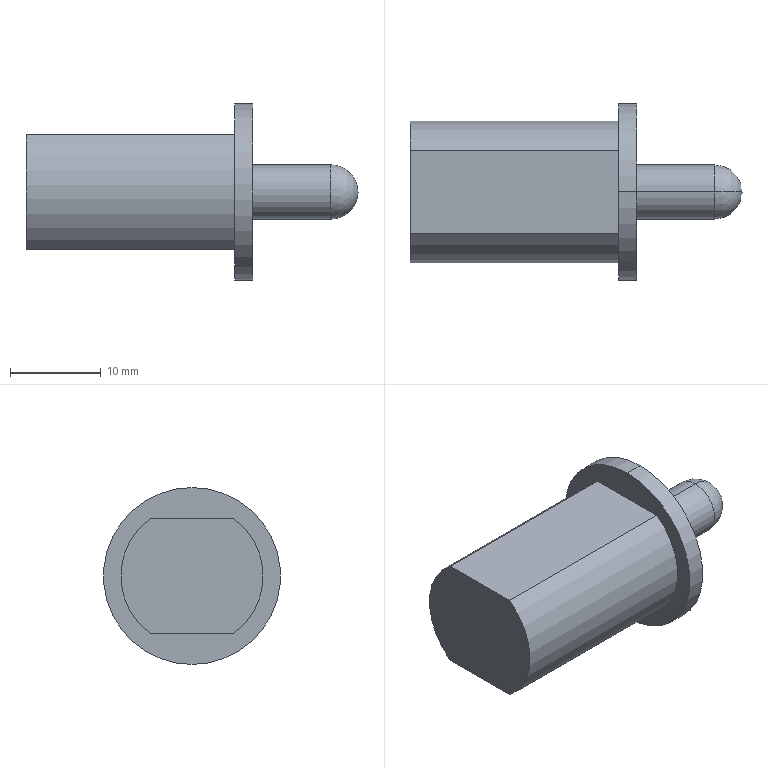Part | STEP file | ZK-0092_160001 | 1 solid | 13 faces | box 36.6 x 19.5 x 19.5 mm | volume 4916 mm3 | cylinder 6 | plane 5 | sphere 2 | commonest cylinder face diameters 6 x2 15.7 x2 19.5 x2
STEP:
#1=CARTESIAN_POINT('',(0.,0.,0.));
#2=DIRECTION('',(0.,0.,1.));
#3=DIRECTION('',(1.,0.,0.));
#4=AXIS2_PLACEMENT_3D('',#1,#2,#3);
#5=CARTESIAN_POINT('',(574.,109.892,1931.35));
#6=VERTEX_POINT('',#5);
#7=CARTESIAN_POINT('',(574.,109.892,1918.65));
#8=VERTEX_POINT('',#7);
#9=CARTESIAN_POINT('',(574.,114.508,1925.));
#10=DIRECTION('',(1.,0.,0.));
#11=DIRECTION('',(0.,-0.5879,0.8089));
#12=AXIS2_PLACEMENT_3D('',#9,#10,#11);
#13=CIRCLE('',#12,7.85);
#14=CARTESIAN_POINT('',(548.,114.508,1925.));
#15=DIRECTION('',(1.,0.,0.));
#16=DIRECTION('',(0.,0.,1.));
#17=AXIS2_PLACEMENT_3D('',#14,#15,#16);
#18=CYLINDRICAL_SURFACE('',#17,7.85);
#19=CARTESIAN_POINT('',(0.6285,26.));
#20=DIRECTION('',(1.,0.));
#21=VECTOR('',#20,1.);
#22=LINE('',#19,#21);
#23=(GEOMETRIC_REPRESENTATION_CONTEXT(2)PARAMETRIC_REPRESENTATION_CONTEXT()REPRESENTATION_CONTEXT('',''));
#24=DEFINITIONAL_REPRESENTATION('',(#22),#23);
#25=PCURVE('',#18,#24);
#26=CARTESIAN_POINT('',(574.,114.508,1925.));
#27=DIRECTION('',(1.,0.,0.));
#28=DIRECTION('',(0.,0.,1.));
#29=AXIS2_PLACEMENT_3D('',#26,#27,#28);
#30=PLANE('',#29);
#31=CARTESIAN_POINT('',(0.,0.));
#32=DIRECTION('',(0.8089,0.5879));
#33=AXIS2_PLACEMENT_2D('',#31,#32);
#34=CIRCLE('',#33,7.85);
#35=(GEOMETRIC_REPRESENTATION_CONTEXT(2)PARAMETRIC_REPRESENTATION_CONTEXT()REPRESENTATION_CONTEXT('',''));
#36=DEFINITIONAL_REPRESENTATION('',(#34),#35);
#37=PCURVE('',#30,#36);
#38=SURFACE_CURVE('',#13,(#25,#37),.PCURVE_S1.);
#39=EDGE_CURVE('',#6,#8,#38,.T.);
#40=ORIENTED_EDGE('',*,*,#39,.F.);
#41=CARTESIAN_POINT('',(551.,109.892,1931.35));
#42=VERTEX_POINT('',#41);
#43=CARTESIAN_POINT('',(574.,109.892,1931.35));
#44=DIRECTION('',(-1.,0.,0.));
#45=VECTOR('',#44,1.);
#46=LINE('',#43,#45);
#47=CARTESIAN_POINT('',(0.6285,26.));
#48=DIRECTION('',(0.,-1.));
#49=VECTOR('',#48,1.);
#50=LINE('',#47,#49);
#51=(GEOMETRIC_REPRESENTATION_CONTEXT(2)PARAMETRIC_REPRESENTATION_CONTEXT()REPRESENTATION_CONTEXT('',''));
#52=DEFINITIONAL_REPRESENTATION('',(#50),#51);
#53=PCURVE('',#18,#52);
#54=CARTESIAN_POINT('',(561.,128.108,1931.35));
#55=DIRECTION('',(0.,0.,-1.));
#56=DIRECTION('',(1.,0.,0.));
#57=AXIS2_PLACEMENT_3D('',#54,#55,#56);
#58=PLANE('',#57);
#59=CARTESIAN_POINT('',(13.,18.215));
#60=DIRECTION('',(-1.,0.));
#61=VECTOR('',#60,1.);
#62=LINE('',#59,#61);
#63=(GEOMETRIC_REPRESENTATION_CONTEXT(2)PARAMETRIC_REPRESENTATION_CONTEXT()REPRESENTATION_CONTEXT('',''));
#64=DEFINITIONAL_REPRESENTATION('',(#62),#63);
#65=PCURVE('',#58,#64);
#66=SURFACE_CURVE('',#46,(#53,#65),.PCURVE_S1.);
#67=EDGE_CURVE('',#6,#42,#66,.T.);
#68=ORIENTED_EDGE('',*,*,#67,.T.);
#69=CARTESIAN_POINT('',(551.,109.892,1918.65));
#70=VERTEX_POINT('',#69);
#71=CARTESIAN_POINT('',(551.,114.508,1925.));
#72=DIRECTION('',(-1.,0.,0.));
#73=DIRECTION('',(0.,-0.5879,-0.8089));
#74=AXIS2_PLACEMENT_3D('',#71,#72,#73);
#75=CIRCLE('',#74,7.85);
#76=CARTESIAN_POINT('',(2.513,3.));
#77=DIRECTION('',(-1.,0.));
#78=VECTOR('',#77,1.);
#79=LINE('',#76,#78);
#80=(GEOMETRIC_REPRESENTATION_CONTEXT(2)PARAMETRIC_REPRESENTATION_CONTEXT()REPRESENTATION_CONTEXT('',''));
#81=DEFINITIONAL_REPRESENTATION('',(#79),#80);
#82=PCURVE('',#18,#81);
#83=CARTESIAN_POINT('',(551.,114.508,1925.));
#84=DIRECTION('',(-1.,0.,0.));
#85=DIRECTION('',(0.,0.,-1.));
#86=AXIS2_PLACEMENT_3D('',#83,#84,#85);
#87=PLANE('',#86);
#88=CARTESIAN_POINT('',(0.,0.));
#89=DIRECTION('',(0.8089,0.5879));
#90=AXIS2_PLACEMENT_2D('',#88,#89);
#91=CIRCLE('',#90,7.85);
#92=(GEOMETRIC_REPRESENTATION_CONTEXT(2)PARAMETRIC_REPRESENTATION_CONTEXT()REPRESENTATION_CONTEXT('',''));
#93=DEFINITIONAL_REPRESENTATION('',(#91),#92);
#94=PCURVE('',#87,#93);
#95=SURFACE_CURVE('',#75,(#82,#94),.PCURVE_S1.);
#96=EDGE_CURVE('',#70,#42,#95,.T.);
#97=ORIENTED_EDGE('',*,*,#96,.F.);
#98=CARTESIAN_POINT('',(551.,109.892,1918.65));
#99=DIRECTION('',(1.,0.,0.));
#100=VECTOR('',#99,1.);
#101=LINE('',#98,#100);
#102=CARTESIAN_POINT('',(2.513,3.));
#103=DIRECTION('',(0.,1.));
#104=VECTOR('',#103,1.);
#105=LINE('',#102,#104);
#106=(GEOMETRIC_REPRESENTATION_CONTEXT(2)PARAMETRIC_REPRESENTATION_CONTEXT()REPRESENTATION_CONTEXT('',''));
#107=DEFINITIONAL_REPRESENTATION('',(#105),#106);
#108=PCURVE('',#18,#107);
#109=CARTESIAN_POINT('',(561.,101.108,1918.65));
#110=DIRECTION('',(0.,0.,1.));
#111=DIRECTION('',(-1.,0.,0.));
#112=AXIS2_PLACEMENT_3D('',#109,#110,#111);
#113=PLANE('',#112);
#114=CARTESIAN_POINT('',(10.,-8.785));
#115=DIRECTION('',(-1.,0.));
#116=VECTOR('',#115,1.);
#117=LINE('',#114,#116);
#118=(GEOMETRIC_REPRESENTATION_CONTEXT(2)PARAMETRIC_REPRESENTATION_CONTEXT()REPRESENTATION_CONTEXT('',''));
#119=DEFINITIONAL_REPRESENTATION('',(#117),#118);
#120=PCURVE('',#113,#119);
#121=SURFACE_CURVE('',#101,(#108,#120),.PCURVE_S1.);
#122=EDGE_CURVE('',#70,#8,#121,.T.);
#123=ORIENTED_EDGE('',*,*,#122,.T.);
#124=EDGE_LOOP('',(#40,#68,#97,#123));
#125=FACE_BOUND('',#124,.T.);
#126=ADVANCED_FACE('',(#125),#18,.T.);
#127=CARTESIAN_POINT('',(551.,119.123,1918.65));
#128=VERTEX_POINT('',#127);
#129=CARTESIAN_POINT('',(551.,119.123,1918.65));
#130=DIRECTION('',(0.,-1.,0.));
#131=VECTOR('',#130,1.);
#132=LINE('',#129,#131);
#133=CARTESIAN_POINT('',(10.,-18.015));
#134=DIRECTION('',(0.,1.));
#135=VECTOR('',#134,1.);
#136=LINE('',#133,#135);
#137=(GEOMETRIC_REPRESENTATION_CONTEXT(2)PARAMETRIC_REPRESENTATION_CONTEXT()REPRESENTATION_CONTEXT('',''));
#138=DEFINITIONAL_REPRESENTATION('',(#136),#137);
#139=PCURVE('',#113,#138);
#140=CARTESIAN_POINT('',(6.35,-4.615));
#141=DIRECTION('',(0.,1.));
#142=VECTOR('',#141,1.);
#143=LINE('',#140,#142);
#144=(GEOMETRIC_REPRESENTATION_CONTEXT(2)PARAMETRIC_REPRESENTATION_CONTEXT()REPRESENTATION_CONTEXT('',''));
#145=DEFINITIONAL_REPRESENTATION('',(#143),#144);
#146=PCURVE('',#87,#145);
#147=SURFACE_CURVE('',#132,(#139,#146),.PCURVE_S1.);
#148=EDGE_CURVE('',#128,#70,#147,.T.);
#149=ORIENTED_EDGE('',*,*,#148,.T.);
#150=ORIENTED_EDGE('',*,*,#122,.T.);
#151=CARTESIAN_POINT('',(574.,119.123,1918.65));
#152=VERTEX_POINT('',#151);
#153=CARTESIAN_POINT('',(574.,109.892,1918.65));
#154=DIRECTION('',(0.,1.,0.));
#155=VECTOR('',#154,1.);
#156=LINE('',#153,#155);
#157=CARTESIAN_POINT('',(-13.,-8.785));
#158=DIRECTION('',(0.,-1.));
#159=VECTOR('',#158,1.);
#160=LINE('',#157,#159);
#161=(GEOMETRIC_REPRESENTATION_CONTEXT(2)PARAMETRIC_REPRESENTATION_CONTEXT()REPRESENTATION_CONTEXT('',''));
#162=DEFINITIONAL_REPRESENTATION('',(#160),#161);
#163=PCURVE('',#113,#162);
#164=CARTESIAN_POINT('',(-6.35,4.615));
#165=DIRECTION('',(0.,-1.));
#166=VECTOR('',#165,1.);
#167=LINE('',#164,#166);
#168=(GEOMETRIC_REPRESENTATION_CONTEXT(2)PARAMETRIC_REPRESENTATION_CONTEXT()REPRESENTATION_CONTEXT('',''));
#169=DEFINITIONAL_REPRESENTATION('',(#167),#168);
#170=PCURVE('',#30,#169);
#171=SURFACE_CURVE('',#156,(#163,#170),.PCURVE_S1.);
#172=EDGE_CURVE('',#8,#152,#171,.T.);
#173=ORIENTED_EDGE('',*,*,#172,.T.);
#174=CARTESIAN_POINT('',(574.,119.123,1918.65));
#175=DIRECTION('',(-1.,0.,0.));
#176=VECTOR('',#175,1.);
#177=LINE('',#174,#176);
#178=CARTESIAN_POINT('',(-13.,-18.015));
#179=DIRECTION('',(1.,0.));
#180=VECTOR('',#179,1.);
#181=LINE('',#178,#180);
#182=(GEOMETRIC_REPRESENTATION_CONTEXT(2)PARAMETRIC_REPRESENTATION_CONTEXT()REPRESENTATION_CONTEXT('',''));
#183=DEFINITIONAL_REPRESENTATION('',(#181),#182);
#184=PCURVE('',#113,#183);
#185=CARTESIAN_POINT('',(548.,114.508,1925.));
#186=DIRECTION('',(1.,0.,0.));
#187=DIRECTION('',(0.,0.,1.));
#188=AXIS2_PLACEMENT_3D('',#185,#186,#187);
#189=CYLINDRICAL_SURFACE('',#188,7.85);
#190=CARTESIAN_POINT('',(3.77,26.));
#191=DIRECTION('',(0.,-1.));
#192=VECTOR('',#191,1.);
#193=LINE('',#190,#192);
#194=(GEOMETRIC_REPRESENTATION_CONTEXT(2)PARAMETRIC_REPRESENTATION_CONTEXT()REPRESENTATION_CONTEXT('',''));
#195=DEFINITIONAL_REPRESENTATION('',(#193),#194);
#196=PCURVE('',#189,#195);
#197=SURFACE_CURVE('',#177,(#184,#196),.PCURVE_S1.);
#198=EDGE_CURVE('',#152,#128,#197,.T.);
#199=ORIENTED_EDGE('',*,*,#198,.T.);
#200=EDGE_LOOP('',(#149,#150,#173,#199));
#201=FACE_BOUND('',#200,.F.);
#202=ADVANCED_FACE('',(#201),#113,.F.);
#203=CARTESIAN_POINT('',(551.,119.123,1931.35));
#204=VERTEX_POINT('',#203);
#205=CARTESIAN_POINT('',(551.,109.892,1931.35));
#206=DIRECTION('',(0.,1.,0.));
#207=VECTOR('',#206,1.);
#208=LINE('',#205,#207);
#209=CARTESIAN_POINT('',(-6.35,4.615));
#210=DIRECTION('',(0.,-1.));
#211=VECTOR('',#210,1.);
#212=LINE('',#209,#211);
#213=(GEOMETRIC_REPRESENTATION_CONTEXT(2)PARAMETRIC_REPRESENTATION_CONTEXT()REPRESENTATION_CONTEXT('',''));
#214=DEFINITIONAL_REPRESENTATION('',(#212),#213);
#215=PCURVE('',#87,#214);
#216=CARTESIAN_POINT('',(-10.,18.215));
#217=DIRECTION('',(0.,-1.));
#218=VECTOR('',#217,1.);
#219=LINE('',#216,#218);
#220=(GEOMETRIC_REPRESENTATION_CONTEXT(2)PARAMETRIC_REPRESENTATION_CONTEXT()REPRESENTATION_CONTEXT('',''));
#221=DEFINITIONAL_REPRESENTATION('',(#219),#220);
#222=PCURVE('',#58,#221);
#223=SURFACE_CURVE('',#208,(#215,#222),.PCURVE_S1.);
#224=EDGE_CURVE('',#42,#204,#223,.T.);
#225=ORIENTED_EDGE('',*,*,#224,.F.);
#226=ORIENTED_EDGE('',*,*,#96,.F.);
#227=ORIENTED_EDGE('',*,*,#148,.F.);
#228=CARTESIAN_POINT('',(551.,114.508,1925.));
#229=DIRECTION('',(-1.,0.,0.));
#230=DIRECTION('',(0.,0.5879,0.8089));
#231=AXIS2_PLACEMENT_3D('',#228,#229,#230);
#232=CIRCLE('',#231,7.85);
#233=CARTESIAN_POINT('',(0.,0.));
#234=DIRECTION('',(-0.8089,-0.5879));
#235=AXIS2_PLACEMENT_2D('',#233,#234);
#236=CIRCLE('',#235,7.85);
#237=(GEOMETRIC_REPRESENTATION_CONTEXT(2)PARAMETRIC_REPRESENTATION_CONTEXT()REPRESENTATION_CONTEXT('',''));
#238=DEFINITIONAL_REPRESENTATION('',(#236),#237);
#239=PCURVE('',#87,#238);
#240=CARTESIAN_POINT('',(5.655,3.));
#241=DIRECTION('',(-1.,0.));
#242=VECTOR('',#241,1.);
#243=LINE('',#240,#242);
#244=(GEOMETRIC_REPRESENTATION_CONTEXT(2)PARAMETRIC_REPRESENTATION_CONTEXT()REPRESENTATION_CONTEXT('',''));
#245=DEFINITIONAL_REPRESENTATION('',(#243),#244);
#246=PCURVE('',#189,#245);
#247=SURFACE_CURVE('',#232,(#239,#246),.PCURVE_S1.);
#248=EDGE_CURVE('',#204,#128,#247,.T.);
#249=ORIENTED_EDGE('',*,*,#248,.F.);
#250=EDGE_LOOP('',(#225,#226,#227,#249));
#251=FACE_BOUND('',#250,.F.);
#252=ADVANCED_FACE('',(#251),#87,.T.);
#253=ORIENTED_EDGE('',*,*,#224,.T.);
#254=CARTESIAN_POINT('',(574.,119.123,1931.35));
#255=VERTEX_POINT('',#254);
#256=CARTESIAN_POINT('',(551.,119.123,1931.35));
#257=DIRECTION('',(1.,0.,0.));
#258=VECTOR('',#257,1.);
#259=LINE('',#256,#258);
#260=CARTESIAN_POINT('',(-10.,8.985));
#261=DIRECTION('',(1.,0.));
#262=VECTOR('',#261,1.);
#263=LINE('',#260,#262);
#264=(GEOMETRIC_REPRESENTATION_CONTEXT(2)PARAMETRIC_REPRESENTATION_CONTEXT()REPRESENTATION_CONTEXT('',''));
#265=DEFINITIONAL_REPRESENTATION('',(#263),#264);
#266=PCURVE('',#58,#265);
#267=CARTESIAN_POINT('',(5.655,3.));
#268=DIRECTION('',(0.,1.));
#269=VECTOR('',#268,1.);
#270=LINE('',#267,#269);
#271=(GEOMETRIC_REPRESENTATION_CONTEXT(2)PARAMETRIC_REPRESENTATION_CONTEXT()REPRESENTATION_CONTEXT('',''));
#272=DEFINITIONAL_REPRESENTATION('',(#270),#271);
#273=PCURVE('',#189,#272);
#274=SURFACE_CURVE('',#259,(#266,#273),.PCURVE_S1.);
#275=EDGE_CURVE('',#204,#255,#274,.T.);
#276=ORIENTED_EDGE('',*,*,#275,.T.);
#277=CARTESIAN_POINT('',(574.,119.123,1931.35));
#278=DIRECTION('',(0.,-1.,0.));
#279=VECTOR('',#278,1.);
#280=LINE('',#277,#279);
#281=CARTESIAN_POINT('',(13.,8.985));
#282=DIRECTION('',(0.,1.));
#283=VECTOR('',#282,1.);
#284=LINE('',#281,#283);
#285=(GEOMETRIC_REPRESENTATION_CONTEXT(2)PARAMETRIC_REPRESENTATION_CONTEXT()REPRESENTATION_CONTEXT('',''));
#286=DEFINITIONAL_REPRESENTATION('',(#284),#285);
#287=PCURVE('',#58,#286);
#288=CARTESIAN_POINT('',(6.35,-4.615));
#289=DIRECTION('',(0.,1.));
#290=VECTOR('',#289,1.);
#291=LINE('',#288,#290);
#292=(GEOMETRIC_REPRESENTATION_CONTEXT(2)PARAMETRIC_REPRESENTATION_CONTEXT()REPRESENTATION_CONTEXT('',''));
#293=DEFINITIONAL_REPRESENTATION('',(#291),#292);
#294=PCURVE('',#30,#293);
#295=SURFACE_CURVE('',#280,(#287,#294),.PCURVE_S1.);
#296=EDGE_CURVE('',#255,#6,#295,.T.);
#297=ORIENTED_EDGE('',*,*,#296,.T.);
#298=ORIENTED_EDGE('',*,*,#67,.T.);
#299=EDGE_LOOP('',(#253,#276,#297,#298));
#300=FACE_BOUND('',#299,.F.);
#301=ADVANCED_FACE('',(#300),#58,.F.);
#302=ORIENTED_EDGE('',*,*,#275,.T.);
#303=CARTESIAN_POINT('',(574.,114.508,1925.));
#304=DIRECTION('',(1.,0.,0.));
#305=DIRECTION('',(0.,0.5879,-0.8089));
#306=AXIS2_PLACEMENT_3D('',#303,#304,#305);
#307=CIRCLE('',#306,7.85);
#308=CARTESIAN_POINT('',(3.77,26.));
#309=DIRECTION('',(1.,0.));
#310=VECTOR('',#309,1.);
#311=LINE('',#308,#310);
#312=(GEOMETRIC_REPRESENTATION_CONTEXT(2)PARAMETRIC_REPRESENTATION_CONTEXT()REPRESENTATION_CONTEXT('',''));
#313=DEFINITIONAL_REPRESENTATION('',(#311),#312);
#314=PCURVE('',#189,#313);
#315=CARTESIAN_POINT('',(0.,0.));
#316=DIRECTION('',(-0.8089,-0.5879));
#317=AXIS2_PLACEMENT_2D('',#315,#316);
#318=CIRCLE('',#317,7.85);
#319=(GEOMETRIC_REPRESENTATION_CONTEXT(2)PARAMETRIC_REPRESENTATION_CONTEXT()REPRESENTATION_CONTEXT('',''));
#320=DEFINITIONAL_REPRESENTATION('',(#318),#319);
#321=PCURVE('',#30,#320);
#322=SURFACE_CURVE('',#307,(#314,#321),.PCURVE_S1.);
#323=EDGE_CURVE('',#152,#255,#322,.T.);
#324=ORIENTED_EDGE('',*,*,#323,.F.);
#325=ORIENTED_EDGE('',*,*,#198,.T.);
#326=ORIENTED_EDGE('',*,*,#248,.F.);
#327=EDGE_LOOP('',(#302,#324,#325,#326));
#328=FACE_BOUND('',#327,.T.);
#329=ADVANCED_FACE('',(#328),#189,.T.);
#330=CARTESIAN_POINT('',(574.,114.508,1915.25));
#331=VERTEX_POINT('',#330);
#332=CARTESIAN_POINT('',(574.,114.508,1934.75));
#333=VERTEX_POINT('',#332);
#334=CARTESIAN_POINT('',(574.,114.508,1925.));
#335=DIRECTION('',(-1.,0.,0.));
#336=DIRECTION('',(0.,0.,-1.));
#337=AXIS2_PLACEMENT_3D('',#334,#335,#336);
#338=CIRCLE('',#337,9.75);
#339=CARTESIAN_POINT('',(-9.75,0.));
#340=CARTESIAN_POINT('',(-9.75,16.887));
#341=CARTESIAN_POINT('',(4.875,8.444));
#342=CARTESIAN_POINT('',(19.5,0.));
#343=CARTESIAN_POINT('',(4.875,-8.444));
#344=CARTESIAN_POINT('',(-9.75,-16.887));
#345=CARTESIAN_POINT('',(-9.75,0.));
#346=(BOUNDED_CURVE()B_SPLINE_CURVE(2,(#339,#340,#341,#342,#343,#344,#345),.UNSPECIFIED.,.T.,.F.)B_SPLINE_CURVE_WITH_KNOTS((1,2,2,2,2,1),(-2.094,0.,2.094,4.189,6.283,8.378),.UNSPECIFIED.)CURVE()GEOMETRIC_REPRESENTATION_ITEM()RATIONAL_B_SPLINE_CURVE((1.,0.5,1.,0.5,1.,0.5,1.))REPRESENTATION_ITEM(''));
#347=(GEOMETRIC_REPRESENTATION_CONTEXT(2)PARAMETRIC_REPRESENTATION_CONTEXT()REPRESENTATION_CONTEXT('',''));
#348=DEFINITIONAL_REPRESENTATION('',(#346),#347);
#349=PCURVE('',#30,#348);
#350=CARTESIAN_POINT('',(576.,114.508,1925.));
#351=DIRECTION('',(-1.,0.,0.));
#352=DIRECTION('',(0.,0.,-1.));
#353=AXIS2_PLACEMENT_3D('',#350,#351,#352);
#354=CYLINDRICAL_SURFACE('',#353,9.75);
#355=CARTESIAN_POINT('',(0.,2.));
#356=DIRECTION('',(1.,0.));
#357=VECTOR('',#356,1.);
#358=LINE('',#355,#357);
#359=(GEOMETRIC_REPRESENTATION_CONTEXT(2)PARAMETRIC_REPRESENTATION_CONTEXT()REPRESENTATION_CONTEXT('',''));
#360=DEFINITIONAL_REPRESENTATION('',(#358),#359);
#361=PCURVE('',#354,#360);
#362=SURFACE_CURVE('',#338,(#349,#361),.PCURVE_S1.);
#363=EDGE_CURVE('',#331,#333,#362,.T.);
#364=ORIENTED_EDGE('',*,*,#363,.F.);
#365=CARTESIAN_POINT('',(574.,114.508,1925.));
#366=DIRECTION('',(-1.,0.,0.));
#367=DIRECTION('',(0.,0.,1.));
#368=AXIS2_PLACEMENT_3D('',#365,#366,#367);
#369=CIRCLE('',#368,9.75);
#370=CARTESIAN_POINT('',(9.75,0.));
#371=CARTESIAN_POINT('',(9.75,-16.887));
#372=CARTESIAN_POINT('',(-4.875,-8.444));
#373=CARTESIAN_POINT('',(-19.5,0.));
#374=CARTESIAN_POINT('',(-4.875,8.444));
#375=CARTESIAN_POINT('',(9.75,16.887));
#376=CARTESIAN_POINT('',(9.75,0.));
#377=(BOUNDED_CURVE()B_SPLINE_CURVE(2,(#370,#371,#372,#373,#374,#375,#376),.UNSPECIFIED.,.T.,.F.)B_SPLINE_CURVE_WITH_KNOTS((1,2,2,2,2,1),(-2.094,0.,2.094,4.189,6.283,8.378),.UNSPECIFIED.)CURVE()GEOMETRIC_REPRESENTATION_ITEM()RATIONAL_B_SPLINE_CURVE((1.,0.5,1.,0.5,1.,0.5,1.))REPRESENTATION_ITEM(''));
#378=(GEOMETRIC_REPRESENTATION_CONTEXT(2)PARAMETRIC_REPRESENTATION_CONTEXT()REPRESENTATION_CONTEXT('',''));
#379=DEFINITIONAL_REPRESENTATION('',(#377),#378);
#380=PCURVE('',#30,#379);
#381=CARTESIAN_POINT('',(576.,114.508,1925.));
#382=DIRECTION('',(-1.,0.,0.));
#383=DIRECTION('',(0.,0.,-1.));
#384=AXIS2_PLACEMENT_3D('',#381,#382,#383);
#385=CYLINDRICAL_SURFACE('',#384,9.75);
#386=CARTESIAN_POINT('',(3.142,2.));
#387=DIRECTION('',(1.,0.));
#388=VECTOR('',#387,1.);
#389=LINE('',#386,#388);
#390=(GEOMETRIC_REPRESENTATION_CONTEXT(2)PARAMETRIC_REPRESENTATION_CONTEXT()REPRESENTATION_CONTEXT('',''));
#391=DEFINITIONAL_REPRESENTATION('',(#389),#390);
#392=PCURVE('',#385,#391);
#393=SURFACE_CURVE('',#369,(#380,#392),.PCURVE_S1.);
#394=EDGE_CURVE('',#333,#331,#393,.T.);
#395=ORIENTED_EDGE('',*,*,#394,.F.);
#396=EDGE_LOOP('',(#364,#395));
#397=FACE_BOUND('',#396,.F.);
#398=ORIENTED_EDGE('',*,*,#323,.F.);
#399=ORIENTED_EDGE('',*,*,#172,.F.);
#400=ORIENTED_EDGE('',*,*,#39,.F.);
#401=ORIENTED_EDGE('',*,*,#296,.F.);
#402=EDGE_LOOP('',(#398,#399,#400,#401));
#403=FACE_BOUND('',#402,.F.);
#404=ADVANCED_FACE('',(#397,#403),#30,.F.);
#405=CARTESIAN_POINT('',(576.,114.508,1934.75));
#406=VERTEX_POINT('',#405);
#407=CARTESIAN_POINT('',(576.,114.508,1934.75));
#408=DIRECTION('',(-1.,0.,0.));
#409=VECTOR('',#408,1.);
#410=LINE('',#407,#409);
#411=CARTESIAN_POINT('',(3.142,0.));
#412=DIRECTION('',(0.,1.));
#413=VECTOR('',#412,1.);
#414=LINE('',#411,#413);
#415=(GEOMETRIC_REPRESENTATION_CONTEXT(2)PARAMETRIC_REPRESENTATION_CONTEXT()REPRESENTATION_CONTEXT('',''));
#416=DEFINITIONAL_REPRESENTATION('',(#414),#415);
#417=PCURVE('',#354,#416);
#418=CARTESIAN_POINT('',(3.142,0.));
#419=DIRECTION('',(0.,1.));
#420=VECTOR('',#419,1.);
#421=LINE('',#418,#420);
#422=(GEOMETRIC_REPRESENTATION_CONTEXT(2)PARAMETRIC_REPRESENTATION_CONTEXT()REPRESENTATION_CONTEXT('',''));
#423=DEFINITIONAL_REPRESENTATION('',(#421),#422);
#424=PCURVE('',#385,#423);
#425=SURFACE_CURVE('',#410,(#417,#424),.PCURVE_S1.);
#426=EDGE_CURVE('',#406,#333,#425,.T.);
#427=ORIENTED_EDGE('',*,*,#426,.T.);
#428=ORIENTED_EDGE('',*,*,#363,.F.);
#429=CARTESIAN_POINT('',(576.,114.508,1915.25));
#430=VERTEX_POINT('',#429);
#431=CARTESIAN_POINT('',(576.,114.508,1915.25));
#432=DIRECTION('',(-1.,0.,0.));
#433=VECTOR('',#432,1.);
#434=LINE('',#431,#433);
#435=CARTESIAN_POINT('',(0.,0.));
#436=DIRECTION('',(0.,1.));
#437=VECTOR('',#436,1.);
#438=LINE('',#435,#437);
#439=(GEOMETRIC_REPRESENTATION_CONTEXT(2)PARAMETRIC_REPRESENTATION_CONTEXT()REPRESENTATION_CONTEXT('',''));
#440=DEFINITIONAL_REPRESENTATION('',(#438),#439);
#441=PCURVE('',#354,#440);
#442=CARTESIAN_POINT('',(6.283,0.));
#443=DIRECTION('',(0.,1.));
#444=VECTOR('',#443,1.);
#445=LINE('',#442,#444);
#446=(GEOMETRIC_REPRESENTATION_CONTEXT(2)PARAMETRIC_REPRESENTATION_CONTEXT()REPRESENTATION_CONTEXT('',''));
#447=DEFINITIONAL_REPRESENTATION('',(#445),#446);
#448=PCURVE('',#385,#447);
#449=SURFACE_CURVE('',#434,(#441,#448),.PCURVE_S1.);
#450=EDGE_CURVE('',#430,#331,#449,.T.);
#451=ORIENTED_EDGE('',*,*,#450,.F.);
#452=CARTESIAN_POINT('',(576.,114.508,1925.));
#453=DIRECTION('',(1.,0.,0.));
#454=DIRECTION('',(0.,0.,1.));
#455=AXIS2_PLACEMENT_3D('',#452,#453,#454);
#456=CIRCLE('',#455,9.75);
#457=CARTESIAN_POINT('',(3.142,0.));
#458=DIRECTION('',(-1.,0.));
#459=VECTOR('',#458,1.);
#460=LINE('',#457,#459);
#461=(GEOMETRIC_REPRESENTATION_CONTEXT(2)PARAMETRIC_REPRESENTATION_CONTEXT()REPRESENTATION_CONTEXT('',''));
#462=DEFINITIONAL_REPRESENTATION('',(#460),#461);
#463=PCURVE('',#354,#462);
#464=CARTESIAN_POINT('',(576.,114.508,1925.));
#465=DIRECTION('',(1.,0.,0.));
#466=DIRECTION('',(0.,0.,1.));
#467=AXIS2_PLACEMENT_3D('',#464,#465,#466);
#468=PLANE('',#467);
#469=CARTESIAN_POINT('',(0.,0.));
#470=DIRECTION('',(1.,0.));
#471=AXIS2_PLACEMENT_2D('',#469,#470);
#472=CIRCLE('',#471,9.75);
#473=(GEOMETRIC_REPRESENTATION_CONTEXT(2)PARAMETRIC_REPRESENTATION_CONTEXT()REPRESENTATION_CONTEXT('',''));
#474=DEFINITIONAL_REPRESENTATION('',(#472),#473);
#475=PCURVE('',#468,#474);
#476=SURFACE_CURVE('',#456,(#463,#475),.PCURVE_S1.);
#477=EDGE_CURVE('',#406,#430,#476,.T.);
#478=ORIENTED_EDGE('',*,*,#477,.F.);
#479=EDGE_LOOP('',(#427,#428,#451,#478));
#480=FACE_BOUND('',#479,.T.);
#481=ADVANCED_FACE('',(#480),#354,.T.);
#482=CARTESIAN_POINT('',(576.,114.508,1925.));
#483=DIRECTION('',(1.,0.,0.));
#484=DIRECTION('',(0.,0.,-1.));
#485=AXIS2_PLACEMENT_3D('',#482,#483,#484);
#486=CIRCLE('',#485,9.75);
#487=CARTESIAN_POINT('',(0.,0.));
#488=DIRECTION('',(-1.,0.));
#489=AXIS2_PLACEMENT_2D('',#487,#488);
#490=CIRCLE('',#489,9.75);
#491=(GEOMETRIC_REPRESENTATION_CONTEXT(2)PARAMETRIC_REPRESENTATION_CONTEXT()REPRESENTATION_CONTEXT('',''));
#492=DEFINITIONAL_REPRESENTATION('',(#490),#491);
#493=PCURVE('',#468,#492);
#494=CARTESIAN_POINT('',(6.283,0.));
#495=DIRECTION('',(-1.,0.));
#496=VECTOR('',#495,1.);
#497=LINE('',#494,#496);
#498=(GEOMETRIC_REPRESENTATION_CONTEXT(2)PARAMETRIC_REPRESENTATION_CONTEXT()REPRESENTATION_CONTEXT('',''));
#499=DEFINITIONAL_REPRESENTATION('',(#497),#498);
#500=PCURVE('',#385,#499);
#501=SURFACE_CURVE('',#486,(#493,#500),.PCURVE_S1.);
#502=EDGE_CURVE('',#430,#406,#501,.T.);
#503=ORIENTED_EDGE('',*,*,#502,.F.);
#504=ORIENTED_EDGE('',*,*,#477,.F.);
#505=EDGE_LOOP('',(#503,#504));
#506=FACE_BOUND('',#505,.F.);
#507=CARTESIAN_POINT('',(576.,114.508,1922.));
#508=VERTEX_POINT('',#507);
#509=CARTESIAN_POINT('',(576.,114.508,1928.));
#510=VERTEX_POINT('',#509);
#511=CARTESIAN_POINT('',(576.,114.508,1925.));
#512=DIRECTION('',(-1.,0.,0.));
#513=DIRECTION('',(0.,0.,-1.));
#514=AXIS2_PLACEMENT_3D('',#511,#512,#513);
#515=CIRCLE('',#514,3.);
#516=CARTESIAN_POINT('',(-3.,0.));
#517=CARTESIAN_POINT('',(-3.,5.196));
#518=CARTESIAN_POINT('',(1.5,2.598));
#519=CARTESIAN_POINT('',(6.,0.));
#520=CARTESIAN_POINT('',(1.5,-2.598));
#521=CARTESIAN_POINT('',(-3.,-5.196));
#522=CARTESIAN_POINT('',(-3.,0.));
#523=(BOUNDED_CURVE()B_SPLINE_CURVE(2,(#516,#517,#518,#519,#520,#521,#522),.UNSPECIFIED.,.T.,.F.)B_SPLINE_CURVE_WITH_KNOTS((1,2,2,2,2,1),(-2.094,0.,2.094,4.189,6.283,8.378),.UNSPECIFIED.)CURVE()GEOMETRIC_REPRESENTATION_ITEM()RATIONAL_B_SPLINE_CURVE((1.,0.5,1.,0.5,1.,0.5,1.))REPRESENTATION_ITEM(''));
#524=(GEOMETRIC_REPRESENTATION_CONTEXT(2)PARAMETRIC_REPRESENTATION_CONTEXT()REPRESENTATION_CONTEXT('',''));
#525=DEFINITIONAL_REPRESENTATION('',(#523),#524);
#526=PCURVE('',#468,#525);
#527=CARTESIAN_POINT('',(587.,114.508,1925.));
#528=DIRECTION('',(-1.,0.,0.));
#529=DIRECTION('',(0.,0.,-1.));
#530=AXIS2_PLACEMENT_3D('',#527,#528,#529);
#531=CYLINDRICAL_SURFACE('',#530,3.);
#532=CARTESIAN_POINT('',(0.,11.));
#533=DIRECTION('',(1.,0.));
#534=VECTOR('',#533,1.);
#535=LINE('',#532,#534);
#536=(GEOMETRIC_REPRESENTATION_CONTEXT(2)PARAMETRIC_REPRESENTATION_CONTEXT()REPRESENTATION_CONTEXT('',''));
#537=DEFINITIONAL_REPRESENTATION('',(#535),#536);
#538=PCURVE('',#531,#537);
#539=SURFACE_CURVE('',#515,(#526,#538),.PCURVE_S1.);
#540=EDGE_CURVE('',#508,#510,#539,.T.);
#541=ORIENTED_EDGE('',*,*,#540,.F.);
#542=CARTESIAN_POINT('',(576.,114.508,1925.));
#543=DIRECTION('',(-1.,0.,0.));
#544=DIRECTION('',(0.,0.,1.));
#545=AXIS2_PLACEMENT_3D('',#542,#543,#544);
#546=CIRCLE('',#545,3.);
#547=CARTESIAN_POINT('',(3.,0.));
#548=CARTESIAN_POINT('',(3.,-5.196));
#549=CARTESIAN_POINT('',(-1.5,-2.598));
#550=CARTESIAN_POINT('',(-6.,0.));
#551=CARTESIAN_POINT('',(-1.5,2.598));
#552=CARTESIAN_POINT('',(3.,5.196));
#553=CARTESIAN_POINT('',(3.,0.));
#554=(BOUNDED_CURVE()B_SPLINE_CURVE(2,(#547,#548,#549,#550,#551,#552,#553),.UNSPECIFIED.,.T.,.F.)B_SPLINE_CURVE_WITH_KNOTS((1,2,2,2,2,1),(-2.094,0.,2.094,4.189,6.283,8.378),.UNSPECIFIED.)CURVE()GEOMETRIC_REPRESENTATION_ITEM()RATIONAL_B_SPLINE_CURVE((1.,0.5,1.,0.5,1.,0.5,1.))REPRESENTATION_ITEM(''));
#555=(GEOMETRIC_REPRESENTATION_CONTEXT(2)PARAMETRIC_REPRESENTATION_CONTEXT()REPRESENTATION_CONTEXT('',''));
#556=DEFINITIONAL_REPRESENTATION('',(#554),#555);
#557=PCURVE('',#468,#556);
#558=CARTESIAN_POINT('',(587.,114.508,1925.));
#559=DIRECTION('',(-1.,0.,0.));
#560=DIRECTION('',(0.,0.,-1.));
#561=AXIS2_PLACEMENT_3D('',#558,#559,#560);
#562=CYLINDRICAL_SURFACE('',#561,3.);
#563=CARTESIAN_POINT('',(3.142,11.));
#564=DIRECTION('',(1.,0.));
#565=VECTOR('',#564,1.);
#566=LINE('',#563,#565);
#567=(GEOMETRIC_REPRESENTATION_CONTEXT(2)PARAMETRIC_REPRESENTATION_CONTEXT()REPRESENTATION_CONTEXT('',''));
#568=DEFINITIONAL_REPRESENTATION('',(#566),#567);
#569=PCURVE('',#562,#568);
#570=SURFACE_CURVE('',#546,(#557,#569),.PCURVE_S1.);
#571=EDGE_CURVE('',#510,#508,#570,.T.);
#572=ORIENTED_EDGE('',*,*,#571,.F.);
#573=EDGE_LOOP('',(#541,#572));
#574=FACE_BOUND('',#573,.F.);
#575=ADVANCED_FACE('',(#506,#574),#468,.T.);
#576=CARTESIAN_POINT('',(584.6,114.508,1928.));
#577=VERTEX_POINT('',#576);
#578=CARTESIAN_POINT('',(584.6,114.508,1928.));
#579=DIRECTION('',(-1.,0.,0.));
#580=VECTOR('',#579,1.);
#581=LINE('',#578,#580);
#582=CARTESIAN_POINT('',(3.142,2.4));
#583=DIRECTION('',(0.,1.));
#584=VECTOR('',#583,1.);
#585=LINE('',#582,#584);
#586=(GEOMETRIC_REPRESENTATION_CONTEXT(2)PARAMETRIC_REPRESENTATION_CONTEXT()REPRESENTATION_CONTEXT('',''));
#587=DEFINITIONAL_REPRESENTATION('',(#585),#586);
#588=PCURVE('',#531,#587);
#589=CARTESIAN_POINT('',(3.142,2.4));
#590=DIRECTION('',(0.,1.));
#591=VECTOR('',#590,1.);
#592=LINE('',#589,#591);
#593=(GEOMETRIC_REPRESENTATION_CONTEXT(2)PARAMETRIC_REPRESENTATION_CONTEXT()REPRESENTATION_CONTEXT('',''));
#594=DEFINITIONAL_REPRESENTATION('',(#592),#593);
#595=PCURVE('',#562,#594);
#596=SURFACE_CURVE('',#581,(#588,#595),.PCURVE_S1.);
#597=EDGE_CURVE('',#577,#510,#596,.T.);
#598=ORIENTED_EDGE('',*,*,#597,.T.);
#599=ORIENTED_EDGE('',*,*,#540,.F.);
#600=CARTESIAN_POINT('',(584.6,114.508,1922.));
#601=VERTEX_POINT('',#600);
#602=CARTESIAN_POINT('',(584.6,114.508,1922.));
#603=DIRECTION('',(-1.,0.,0.));
#604=VECTOR('',#603,1.);
#605=LINE('',#602,#604);
#606=CARTESIAN_POINT('',(0.,2.4));
#607=DIRECTION('',(0.,1.));
#608=VECTOR('',#607,1.);
#609=LINE('',#606,#608);
#610=(GEOMETRIC_REPRESENTATION_CONTEXT(2)PARAMETRIC_REPRESENTATION_CONTEXT()REPRESENTATION_CONTEXT('',''));
#611=DEFINITIONAL_REPRESENTATION('',(#609),#610);
#612=PCURVE('',#531,#611);
#613=CARTESIAN_POINT('',(6.283,2.4));
#614=DIRECTION('',(0.,1.));
#615=VECTOR('',#614,1.);
#616=LINE('',#613,#615);
#617=(GEOMETRIC_REPRESENTATION_CONTEXT(2)PARAMETRIC_REPRESENTATION_CONTEXT()REPRESENTATION_CONTEXT('',''));
#618=DEFINITIONAL_REPRESENTATION('',(#616),#617);
#619=PCURVE('',#562,#618);
#620=SURFACE_CURVE('',#605,(#612,#619),.PCURVE_S1.);
#621=EDGE_CURVE('',#601,#508,#620,.T.);
#622=ORIENTED_EDGE('',*,*,#621,.F.);
#623=CARTESIAN_POINT('',(584.6,114.508,1925.));
#624=DIRECTION('',(1.,0.,0.));
#625=DIRECTION('',(0.,0.,1.));
#626=AXIS2_PLACEMENT_3D('',#623,#624,#625);
#627=CIRCLE('',#626,3.);
#628=CARTESIAN_POINT('',(3.142,2.4));
#629=DIRECTION('',(-1.,0.));
#630=VECTOR('',#629,1.);
#631=LINE('',#628,#630);
#632=(GEOMETRIC_REPRESENTATION_CONTEXT(2)PARAMETRIC_REPRESENTATION_CONTEXT()REPRESENTATION_CONTEXT('',''));
#633=DEFINITIONAL_REPRESENTATION('',(#631),#632);
#634=PCURVE('',#531,#633);
#635=CARTESIAN_POINT('',(584.6,114.508,1925.));
#636=DIRECTION('',(1.,0.,0.));
#637=DIRECTION('',(0.,0.,1.));
#638=AXIS2_PLACEMENT_3D('',#635,#636,#637);
#639=SPHERICAL_SURFACE('',#638,3.);
#640=CARTESIAN_POINT('',(0.,0.));
#641=DIRECTION('',(1.,0.));
#642=VECTOR('',#641,1.);
#643=LINE('',#640,#642);
#644=(GEOMETRIC_REPRESENTATION_CONTEXT(2)PARAMETRIC_REPRESENTATION_CONTEXT()REPRESENTATION_CONTEXT('',''));
#645=DEFINITIONAL_REPRESENTATION('',(#643),#644);
#646=PCURVE('',#639,#645);
#647=SURFACE_CURVE('',#627,(#634,#646),.PCURVE_S1.);
#648=EDGE_CURVE('',#577,#601,#647,.T.);
#649=ORIENTED_EDGE('',*,*,#648,.F.);
#650=EDGE_LOOP('',(#598,#599,#622,#649));
#651=FACE_BOUND('',#650,.T.);
#652=ADVANCED_FACE('',(#651),#531,.T.);
#653=CARTESIAN_POINT('',(587.6,114.508,1925.));
#654=VERTEX_POINT('',#653);
#655=CARTESIAN_POINT('',(584.6,114.508,1925.));
#656=DIRECTION('',(0.,-1.,0.));
#657=DIRECTION('',(0.,0.,-1.));
#658=AXIS2_PLACEMENT_3D('',#655,#656,#657);
#659=CIRCLE('',#658,3.);
#660=CARTESIAN_POINT('',(3.142,0.));
#661=CARTESIAN_POINT('',(3.142,0.0238));
#662=CARTESIAN_POINT('',(3.142,0.0714));
#663=CARTESIAN_POINT('',(3.142,0.1428));
#664=CARTESIAN_POINT('',(3.142,0.2142));
#665=CARTESIAN_POINT('',(3.142,0.2856));
#666=CARTESIAN_POINT('',(3.142,0.357));
#667=CARTESIAN_POINT('',(3.142,0.4284));
#668=CARTESIAN_POINT('',(3.142,0.4998));
#669=CARTESIAN_POINT('',(3.142,0.5712));
#670=CARTESIAN_POINT('',(3.142,0.6426));
#671=CARTESIAN_POINT('',(3.142,0.714));
#672=CARTESIAN_POINT('',(3.142,0.7854));
#673=CARTESIAN_POINT('',(3.142,0.8568));
#674=CARTESIAN_POINT('',(3.142,0.9282));
#675=CARTESIAN_POINT('',(3.142,0.9996));
#676=CARTESIAN_POINT('',(3.142,1.071));
#677=CARTESIAN_POINT('',(3.142,1.142));
#678=CARTESIAN_POINT('',(3.142,1.214));
#679=CARTESIAN_POINT('',(3.142,1.285));
#680=CARTESIAN_POINT('',(3.142,1.357));
#681=CARTESIAN_POINT('',(3.142,1.428));
#682=CARTESIAN_POINT('',(3.142,1.499));
#683=CARTESIAN_POINT('',(3.142,1.547));
#684=CARTESIAN_POINT('',(3.142,1.571));
#685=B_SPLINE_CURVE_WITH_KNOTS('',3,(#660,#661,#662,#663,#664,#665,#666,#667,#668,#669,#670,#671,#672,#673,#674,#675,#676,#677,#678,#679,#680,#681,#682,#683,#684),.UNSPECIFIED.,.F.,.F.,(4,1,1,1,1,1,1,1,1,1,1,1,1,1,1,1,1,1,1,1,1,1,4),(0.,0.0714,0.1428,0.2142,0.2856,0.357,0.4284,0.4998,0.5712,0.6426,0.714,0.7854,0.8568,0.9282,0.9996,1.071,1.142,1.214,1.285,1.357,1.428,1.499,1.571),.QUASI_UNIFORM_KNOTS.);
#686=(GEOMETRIC_REPRESENTATION_CONTEXT(2)PARAMETRIC_REPRESENTATION_CONTEXT()REPRESENTATION_CONTEXT('',''));
#687=DEFINITIONAL_REPRESENTATION('',(#685),#686);
#688=PCURVE('',#639,#687);
#689=CARTESIAN_POINT('',(584.6,114.508,1925.));
#690=DIRECTION('',(1.,0.,0.));
#691=DIRECTION('',(0.,0.,1.));
#692=AXIS2_PLACEMENT_3D('',#689,#690,#691);
#693=SPHERICAL_SURFACE('',#692,3.);
#694=CARTESIAN_POINT('',(3.142,0.));
#695=CARTESIAN_POINT('',(3.142,0.0238));
#696=CARTESIAN_POINT('',(3.142,0.0714));
#697=CARTESIAN_POINT('',(3.142,0.1428));
#698=CARTESIAN_POINT('',(3.142,0.2142));
#699=CARTESIAN_POINT('',(3.142,0.2856));
#700=CARTESIAN_POINT('',(3.142,0.357));
#701=CARTESIAN_POINT('',(3.142,0.4284));
#702=CARTESIAN_POINT('',(3.142,0.4998));
#703=CARTESIAN_POINT('',(3.142,0.5712));
#704=CARTESIAN_POINT('',(3.142,0.6426));
#705=CARTESIAN_POINT('',(3.142,0.714));
#706=CARTESIAN_POINT('',(3.142,0.7854));
#707=CARTESIAN_POINT('',(3.142,0.8568));
#708=CARTESIAN_POINT('',(3.142,0.9282));
#709=CARTESIAN_POINT('',(3.142,0.9996));
#710=CARTESIAN_POINT('',(3.142,1.071));
#711=CARTESIAN_POINT('',(3.142,1.142));
#712=CARTESIAN_POINT('',(3.142,1.214));
#713=CARTESIAN_POINT('',(3.142,1.285));
#714=CARTESIAN_POINT('',(3.142,1.357));
#715=CARTESIAN_POINT('',(3.142,1.428));
#716=CARTESIAN_POINT('',(3.142,1.499));
#717=CARTESIAN_POINT('',(3.142,1.547));
#718=CARTESIAN_POINT('',(3.142,1.571));
#719=B_SPLINE_CURVE_WITH_KNOTS('',3,(#694,#695,#696,#697,#698,#699,#700,#701,#702,#703,#704,#705,#706,#707,#708,#709,#710,#711,#712,#713,#714,#715,#716,#717,#718),.UNSPECIFIED.,.F.,.F.,(4,1,1,1,1,1,1,1,1,1,1,1,1,1,1,1,1,1,1,1,1,1,4),(0.,0.0714,0.1428,0.2142,0.2856,0.357,0.4284,0.4998,0.5712,0.6426,0.714,0.7854,0.8568,0.9282,0.9996,1.071,1.142,1.214,1.285,1.357,1.428,1.499,1.571),.QUASI_UNIFORM_KNOTS.);
#720=(GEOMETRIC_REPRESENTATION_CONTEXT(2)PARAMETRIC_REPRESENTATION_CONTEXT()REPRESENTATION_CONTEXT('',''));
#721=DEFINITIONAL_REPRESENTATION('',(#719),#720);
#722=PCURVE('',#693,#721);
#723=SURFACE_CURVE('',#659,(#688,#722),.PCURVE_S1.);
#724=EDGE_CURVE('',#601,#654,#723,.T.);
#725=ORIENTED_EDGE('',*,*,#724,.T.);
#726=CARTESIAN_POINT('',(584.6,114.508,1925.));
#727=DIRECTION('',(0.,1.,0.));
#728=DIRECTION('',(0.,0.,1.));
#729=AXIS2_PLACEMENT_3D('',#726,#727,#728);
#730=CIRCLE('',#729,3.);
#731=CARTESIAN_POINT('',(0.,0.));
#732=DIRECTION('',(0.,1.));
#733=VECTOR('',#732,1.);
#734=LINE('',#731,#733);
#735=(GEOMETRIC_REPRESENTATION_CONTEXT(2)PARAMETRIC_REPRESENTATION_CONTEXT()REPRESENTATION_CONTEXT('',''));
#736=DEFINITIONAL_REPRESENTATION('',(#734),#735);
#737=PCURVE('',#639,#736);
#738=CARTESIAN_POINT('',(6.283,0.));
#739=DIRECTION('',(0.,1.));
#740=VECTOR('',#739,1.);
#741=LINE('',#738,#740);
#742=(GEOMETRIC_REPRESENTATION_CONTEXT(2)PARAMETRIC_REPRESENTATION_CONTEXT()REPRESENTATION_CONTEXT('',''));
#743=DEFINITIONAL_REPRESENTATION('',(#741),#742);
#744=PCURVE('',#693,#743);
#745=SURFACE_CURVE('',#730,(#737,#744),.PCURVE_S1.);
#746=EDGE_CURVE('',#577,#654,#745,.T.);
#747=ORIENTED_EDGE('',*,*,#746,.F.);
#748=ORIENTED_EDGE('',*,*,#648,.T.);
#749=EDGE_LOOP('',(#725,#747,#748));
#750=FACE_BOUND('',#749,.T.);
#751=ADVANCED_FACE('',(#750),#639,.T.);
#752=ORIENTED_EDGE('',*,*,#746,.T.);
#753=ORIENTED_EDGE('',*,*,#724,.F.);
#754=CARTESIAN_POINT('',(584.6,114.508,1925.));
#755=DIRECTION('',(1.,0.,0.));
#756=DIRECTION('',(0.,0.,-1.));
#757=AXIS2_PLACEMENT_3D('',#754,#755,#756);
#758=CIRCLE('',#757,3.);
#759=CARTESIAN_POINT('',(3.142,0.));
#760=CARTESIAN_POINT('',(3.189,0.));
#761=CARTESIAN_POINT('',(3.284,0.));
#762=CARTESIAN_POINT('',(3.427,0.));
#763=CARTESIAN_POINT('',(3.57,0.));
#764=CARTESIAN_POINT('',(3.713,0.));
#765=CARTESIAN_POINT('',(3.856,0.));
#766=CARTESIAN_POINT('',(3.998,0.));
#767=CARTESIAN_POINT('',(4.141,0.));
#768=CARTESIAN_POINT('',(4.284,0.));
#769=CARTESIAN_POINT('',(4.427,0.));
#770=CARTESIAN_POINT('',(4.57,0.));
#771=CARTESIAN_POINT('',(4.712,0.));
#772=CARTESIAN_POINT('',(4.855,0.));
#773=CARTESIAN_POINT('',(4.998,0.));
#774=CARTESIAN_POINT('',(5.141,0.));
#775=CARTESIAN_POINT('',(5.284,0.));
#776=CARTESIAN_POINT('',(5.426,0.));
#777=CARTESIAN_POINT('',(5.569,0.));
#778=CARTESIAN_POINT('',(5.712,0.));
#779=CARTESIAN_POINT('',(5.855,0.));
#780=CARTESIAN_POINT('',(5.998,0.));
#781=CARTESIAN_POINT('',(6.14,0.));
#782=CARTESIAN_POINT('',(6.236,0.));
#783=CARTESIAN_POINT('',(6.283,0.));
#784=B_SPLINE_CURVE_WITH_KNOTS('',3,(#759,#760,#761,#762,#763,#764,#765,#766,#767,#768,#769,#770,#771,#772,#773,#774,#775,#776,#777,#778,#779,#780,#781,#782,#783),.UNSPECIFIED.,.F.,.F.,(4,1,1,1,1,1,1,1,1,1,1,1,1,1,1,1,1,1,1,1,1,1,4),(0.,0.1428,0.2856,0.4284,0.5712,0.714,0.8568,0.9996,1.142,1.285,1.428,1.571,1.714,1.856,1.999,2.142,2.285,2.428,2.57,2.713,2.856,2.999,3.142),.QUASI_UNIFORM_KNOTS.);
#785=(GEOMETRIC_REPRESENTATION_CONTEXT(2)PARAMETRIC_REPRESENTATION_CONTEXT()REPRESENTATION_CONTEXT('',''));
#786=DEFINITIONAL_REPRESENTATION('',(#784),#785);
#787=PCURVE('',#693,#786);
#788=CARTESIAN_POINT('',(6.283,2.4));
#789=DIRECTION('',(-1.,0.));
#790=VECTOR('',#789,1.);
#791=LINE('',#788,#790);
#792=(GEOMETRIC_REPRESENTATION_CONTEXT(2)PARAMETRIC_REPRESENTATION_CONTEXT()REPRESENTATION_CONTEXT('',''));
#793=DEFINITIONAL_REPRESENTATION('',(#791),#792);
#794=PCURVE('',#562,#793);
#795=SURFACE_CURVE('',#758,(#787,#794),.PCURVE_S1.);
#796=EDGE_CURVE('',#601,#577,#795,.T.);
#797=ORIENTED_EDGE('',*,*,#796,.T.);
#798=EDGE_LOOP('',(#752,#753,#797));
#799=FACE_BOUND('',#798,.T.);
#800=ADVANCED_FACE('',(#799),#693,.T.);
#801=ORIENTED_EDGE('',*,*,#621,.T.);
#802=ORIENTED_EDGE('',*,*,#571,.F.);
#803=ORIENTED_EDGE('',*,*,#597,.F.);
#804=ORIENTED_EDGE('',*,*,#796,.F.);
#805=EDGE_LOOP('',(#801,#802,#803,#804));
#806=FACE_BOUND('',#805,.T.);
#807=ADVANCED_FACE('',(#806),#562,.T.);
#808=ORIENTED_EDGE('',*,*,#450,.T.);
#809=ORIENTED_EDGE('',*,*,#394,.F.);
#810=ORIENTED_EDGE('',*,*,#426,.F.);
#811=ORIENTED_EDGE('',*,*,#502,.F.);
#812=EDGE_LOOP('',(#808,#809,#810,#811));
#813=FACE_BOUND('',#812,.T.);
#814=ADVANCED_FACE('',(#813),#385,.T.);
#815=CLOSED_SHELL('',(#126,#202,#252,#301,#329,#404,#481,#575,#652,#751,#800,#807,#814));
#816=MANIFOLD_SOLID_BREP('',#815);
#817=(LENGTH_UNIT()NAMED_UNIT(*)SI_UNIT(.MILLI.,.METRE.));
#818=UNCERTAINTY_MEASURE_WITH_UNIT(LENGTH_MEASURE(0.0000001),#817,'','');
#819=(NAMED_UNIT(*)PLANE_ANGLE_UNIT()SI_UNIT($,.RADIAN.));
#820=(NAMED_UNIT(*)SI_UNIT($,.STERADIAN.)SOLID_ANGLE_UNIT());
#821=(GEOMETRIC_REPRESENTATION_CONTEXT(3)GLOBAL_UNCERTAINTY_ASSIGNED_CONTEXT((#818))GLOBAL_UNIT_ASSIGNED_CONTEXT((#817,#819,#820))REPRESENTATION_CONTEXT('',''));
#822=ADVANCED_BREP_SHAPE_REPRESENTATION('',(#4,#816),#821);